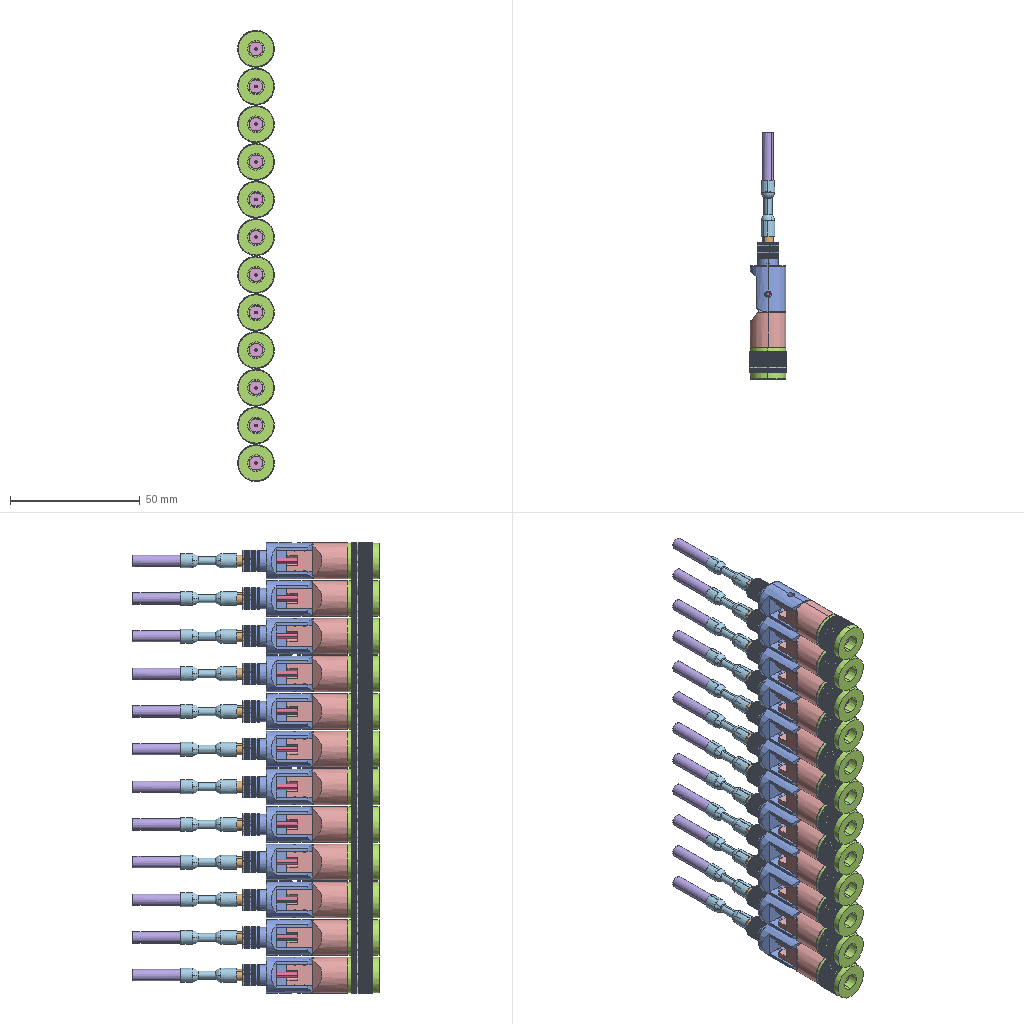Assembly | SolidWorks | 10 different items | 120 placed | box 14 x 95 x 174 mm
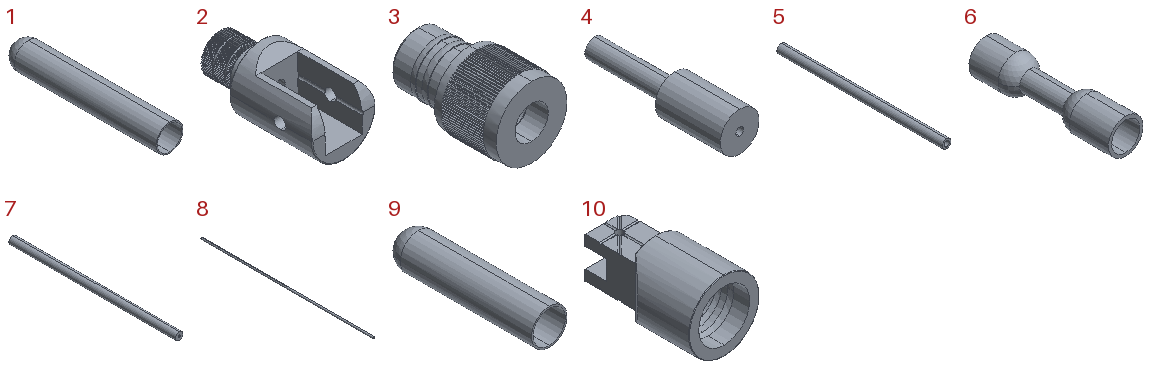Parts list (item | quantity | size | volume | features):
1 | x12 | 4.36 x 24.8 x 4.36 mm | 67.655 mm3 | features Revolution 1
2 | x12 | 13.8 x 26.9 x 13.8 mm | 1584 mm3 | features ICE 7, Fillet 2, CirPattern 1, RevCut 1, Revolution 1
3 | x12 | 14.16 x 22.4 x 14.16 mm | 2205 mm3 | features Chamfer 1, CirPattern 1, ICE 1, Revolution 1
4 | x12 | 5.05 x 18.84 x 5.05 mm | 205.304 mm3 | features Revolution 1
5 | x12 | 1 x 18.84 x 1 mm | 9.47 mm3 | features Revolution 1
6 | x12 | 5.36 x 21.494 x 5.36 mm | 139.623 mm3 | features RevolutionThin 1
7 | x12 | 2.1 x 47 x 2.1 mm | 153.561 mm3 | features Revolution 1
8 | x12 | 0.5 x 48 x 0.5 mm | 9.425 mm3 | features Revolution 1
9 | x12 | 4.36 x 17.91 x 4.36 mm | 48.792 mm3 | features Revolution 1
10 | x12 | 13.8 x 23.5 x 13.8 mm | 1561 mm3 | features ICE 7, Fillet 2, MirrorPattern 1, Revolution 1
Mates (type | each side: item.copy, entity, surface, feature):
Coordinate | 10.1 select_type:25 | assembly select_type:11
Coincident | 2.1 plane | assembly plane
Concentric | 10.1 face cylinder Cut-Extrude3 | 2.1 face cylinder Cut-Extrude8
Concentric | 10.1 face cylinder Revolve1 | 3.1 face cylinder Revolve1
Coincident | 10.1 face plane Revolve1 | 3.1 face plane Revolve1
Concentric | 3.1 face cylinder Revolve1 | 4.1 face cylinder Revolve2
Coincident | 3.1 face plane Revolve1 | 4.1 face plane Revolve2
Concentric | 5.1 face cylinder Revolve2 | 3.1 face cylinder Revolve1
Coincident | 3.1 face plane Revolve1 | 5.1 face plane Revolve2
Concentric | 2.1 face cylinder Revolve1 | 9.1 face cylinder Revolve1
DistanceDim | 9.1 face plane Revolve1 | 2.1 face plane Revolve1
Concentric | 9.1 face cylinder Revolve1 | 1.1 face cylinder Revolve1
DistanceDim | 9.1 face plane Revolve1 | 1.1 face plane Revolve1
Concentric | 10.1 face cylinder Cut-Extrude2 | 8.1 face cylinder Revolve1
Coincident | 5.1 face plane Revolve2 | 8.1 face plane Revolve1
Concentric | 8.1 face cylinder Revolve1 | 7.1 face cylinder Revolve1
Coincident | 4.1 face plane Revolve2 | 7.1 face plane Revolve1
Concentric | 2.1 face cylinder Cut-Extrude1 | 7.1 face cylinder Revolve1
Concentric | 7.1 face cylinder Revolve1 | 6.1 face cylinder Revolve-Thin1
Concentric | 1.1 face sphere Revolve1 | 6.1 face sphere Revolve-Thin1